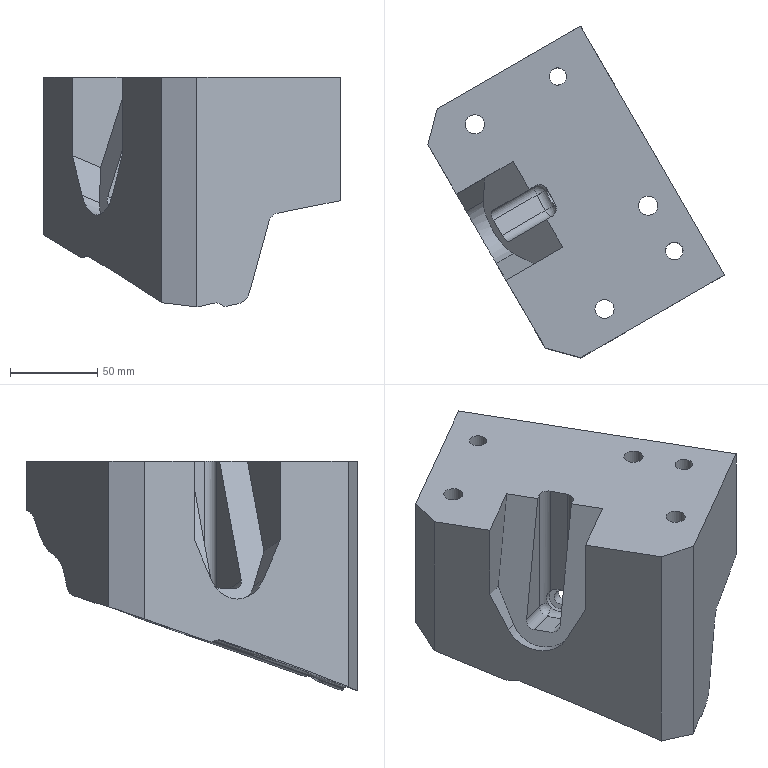Part | NX | features solid 2 | 1 solid | 107 faces | box 170.263 x 190.394 x 131.965 mm | volume 1270035 mm3 | spline 69 | plane 20 | cylinder 16 | sphere 2 | commonest cylinder face diameters 10 x7 11 x3 17 x3 8.1 x1 14 x1 39 x1